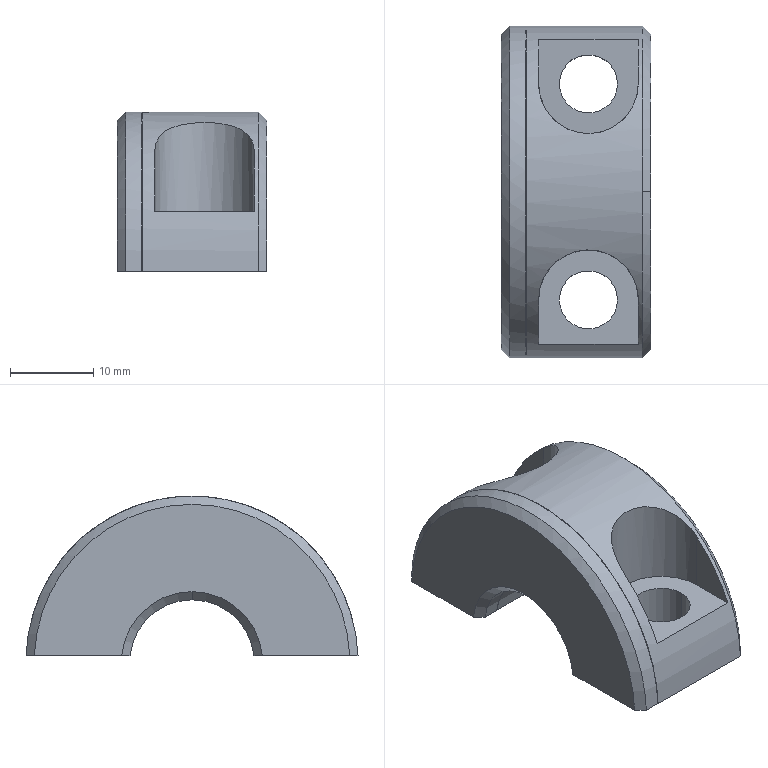Part | STEP file | 0232_Z_SSCSPD15_1 | 1 solid | 31 faces | box 18 x 39.972 x 19.25 mm | volume 7194 mm3 | plane 12 | cylinder 10 | cone 9 | commonest cylinder face diameters 7 x4 12 x2 15 x2 40 x2